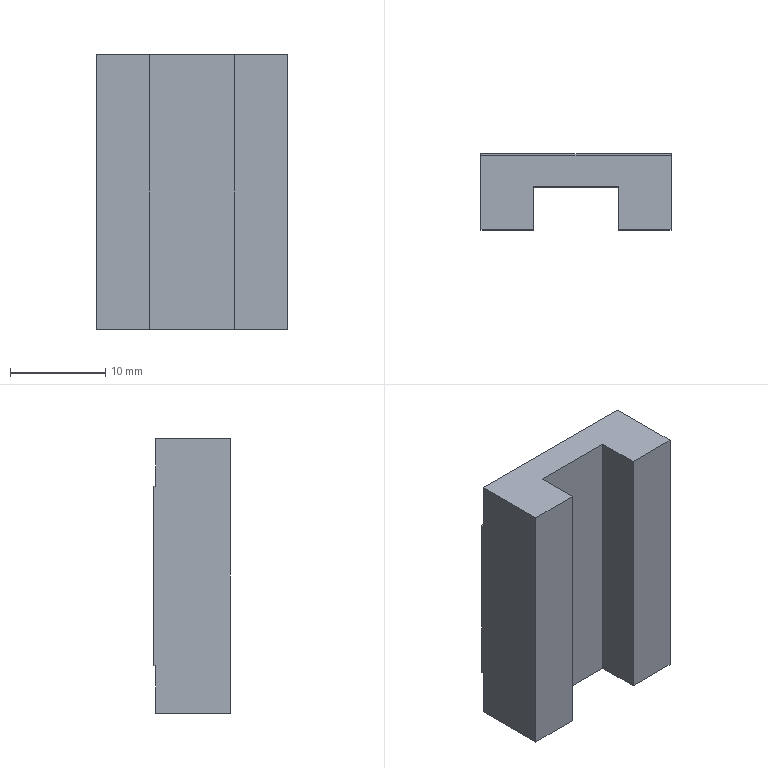Part | STEP file | Mount electronic clip s MGN9C slider | 1 solid | 26 faces | box 20 x 8 x 28.9 mm | volume 3355 mm3 | plane 18 | cylinder 8 | commonest cylinder face diameters 2.5 x8